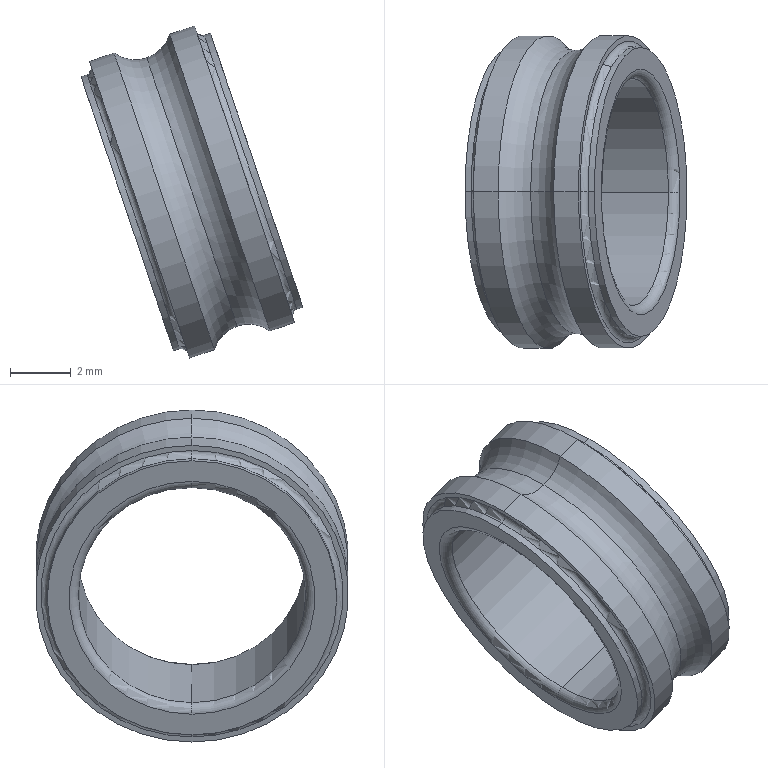Part | STEP file | 2026.6.15-Main Assembly图.sldasm-Part-232 | 1 solid | 26 faces | box 7.316 x 10.32 x 10.946 mm | volume 146.051 mm3 | torus 12 | cylinder 10 | plane 4 | commonest cylinder face diameters 9.54 x4 10.32 x4 7.5 x2